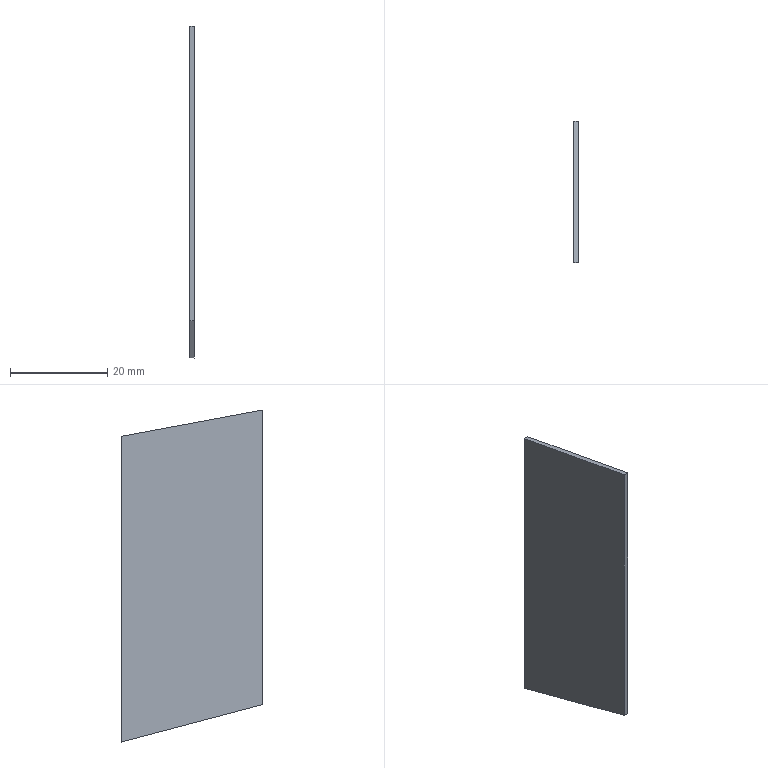Part | STEP file | 09-23 Inlet upper seal plate | 1 solid | 6 faces | box 1 x 29 x 68.181 mm | volume 1787 mm3 | plane 6
STEP:
#1=CARTESIAN_POINT('',(0.,0.,0.));
#2=DIRECTION('',(0.,0.,1.));
#3=DIRECTION('',(1.,0.,0.));
#4=AXIS2_PLACEMENT_3D('',#1,#2,#3);
#5=CARTESIAN_POINT('',(0.,0.,-60.5));
#6=VERTEX_POINT('',#5);
#7=CARTESIAN_POINT('',(1.,0.,-60.5));
#8=VERTEX_POINT('',#7);
#9=CARTESIAN_POINT('',(0.5,0.,-60.5));
#10=DIRECTION('',(1.,0.,0.));
#11=VECTOR('',#10,1.);
#12=LINE('',#9,#11);
#13=CARTESIAN_POINT('',(0.,0.,-60.5));
#14=DIRECTION('',(0.,1.,0.));
#15=DIRECTION('',(0.,0.,1.));
#16=AXIS2_PLACEMENT_3D('',#13,#14,#15);
#17=PLANE('',#16);
#18=CARTESIAN_POINT('',(0.,0.5));
#19=DIRECTION('',(0.,1.));
#20=VECTOR('',#19,1.);
#21=LINE('',#18,#20);
#22=(GEOMETRIC_REPRESENTATION_CONTEXT(2)PARAMETRIC_REPRESENTATION_CONTEXT()REPRESENTATION_CONTEXT('',''));
#23=DEFINITIONAL_REPRESENTATION('',(#21),#22);
#24=PCURVE('',#17,#23);
#25=CARTESIAN_POINT('',(0.,29.,-68.181));
#26=DIRECTION('',(0.,0.256,0.9667));
#27=DIRECTION('',(0.,-0.9667,0.256));
#28=AXIS2_PLACEMENT_3D('',#25,#26,#27);
#29=PLANE('',#28);
#30=CARTESIAN_POINT('',(30.,0.5));
#31=DIRECTION('',(0.,1.));
#32=VECTOR('',#31,1.);
#33=LINE('',#30,#32);
#34=(GEOMETRIC_REPRESENTATION_CONTEXT(2)PARAMETRIC_REPRESENTATION_CONTEXT()REPRESENTATION_CONTEXT('',''));
#35=DEFINITIONAL_REPRESENTATION('',(#33),#34);
#36=PCURVE('',#29,#35);
#37=SURFACE_CURVE('',#12,(#24,#36),.PCURVE_S1.);
#38=EDGE_CURVE('',#6,#8,#37,.T.);
#39=ORIENTED_EDGE('',*,*,#38,.T.);
#40=CARTESIAN_POINT('',(1.,0.,0.));
#41=VERTEX_POINT('',#40);
#42=CARTESIAN_POINT('',(1.,0.,-30.25));
#43=DIRECTION('',(0.,0.,-1.));
#44=VECTOR('',#43,1.);
#45=LINE('',#42,#44);
#46=CARTESIAN_POINT('',(30.25,1.));
#47=DIRECTION('',(-1.,0.));
#48=VECTOR('',#47,1.);
#49=LINE('',#46,#48);
#50=(GEOMETRIC_REPRESENTATION_CONTEXT(2)PARAMETRIC_REPRESENTATION_CONTEXT()REPRESENTATION_CONTEXT('',''));
#51=DEFINITIONAL_REPRESENTATION('',(#49),#50);
#52=PCURVE('',#17,#51);
#53=CARTESIAN_POINT('',(1.,0.,-68.59));
#54=DIRECTION('',(-1.,0.,0.));
#55=DIRECTION('',(0.,0.,1.));
#56=AXIS2_PLACEMENT_3D('',#53,#54,#55);
#57=PLANE('',#56);
#58=CARTESIAN_POINT('',(38.34,0.));
#59=DIRECTION('',(-1.,0.));
#60=VECTOR('',#59,1.);
#61=LINE('',#58,#60);
#62=(GEOMETRIC_REPRESENTATION_CONTEXT(2)PARAMETRIC_REPRESENTATION_CONTEXT()REPRESENTATION_CONTEXT('',''));
#63=DEFINITIONAL_REPRESENTATION('',(#61),#62);
#64=PCURVE('',#57,#63);
#65=SURFACE_CURVE('',#45,(#52,#64),.PCURVE_S1.);
#66=EDGE_CURVE('',#41,#8,#65,.T.);
#67=ORIENTED_EDGE('',*,*,#66,.F.);
#68=CARTESIAN_POINT('',(0.,0.,-0.000000009));
#69=VERTEX_POINT('',#68);
#70=CARTESIAN_POINT('',(0.5,0.,0.));
#71=DIRECTION('',(-1.,0.,0.));
#72=VECTOR('',#71,1.);
#73=LINE('',#70,#72);
#74=CARTESIAN_POINT('',(60.5,0.5));
#75=DIRECTION('',(0.,-1.));
#76=VECTOR('',#75,1.);
#77=LINE('',#74,#76);
#78=(GEOMETRIC_REPRESENTATION_CONTEXT(2)PARAMETRIC_REPRESENTATION_CONTEXT()REPRESENTATION_CONTEXT('',''));
#79=DEFINITIONAL_REPRESENTATION('',(#77),#78);
#80=PCURVE('',#17,#79);
#81=CARTESIAN_POINT('',(0.,0.,0.));
#82=DIRECTION('',(0.,-0.1833,-0.9831));
#83=DIRECTION('',(0.,0.9831,-0.1833));
#84=AXIS2_PLACEMENT_3D('',#81,#82,#83);
#85=PLANE('',#84);
#86=CARTESIAN_POINT('',(0.,0.5));
#87=DIRECTION('',(0.,-1.));
#88=VECTOR('',#87,1.);
#89=LINE('',#86,#88);
#90=(GEOMETRIC_REPRESENTATION_CONTEXT(2)PARAMETRIC_REPRESENTATION_CONTEXT()REPRESENTATION_CONTEXT('',''));
#91=DEFINITIONAL_REPRESENTATION('',(#89),#90);
#92=PCURVE('',#85,#91);
#93=SURFACE_CURVE('',#73,(#80,#92),.PCURVE_S1.);
#94=EDGE_CURVE('',#41,#69,#93,.T.);
#95=ORIENTED_EDGE('',*,*,#94,.T.);
#96=CARTESIAN_POINT('',(0.,0.,-30.25));
#97=DIRECTION('',(0.,0.,1.));
#98=VECTOR('',#97,1.);
#99=LINE('',#96,#98);
#100=CARTESIAN_POINT('',(30.25,0.));
#101=DIRECTION('',(1.,0.));
#102=VECTOR('',#101,1.);
#103=LINE('',#100,#102);
#104=(GEOMETRIC_REPRESENTATION_CONTEXT(2)PARAMETRIC_REPRESENTATION_CONTEXT()REPRESENTATION_CONTEXT('',''));
#105=DEFINITIONAL_REPRESENTATION('',(#103),#104);
#106=PCURVE('',#17,#105);
#107=CARTESIAN_POINT('',(0.,0.,-68.59));
#108=DIRECTION('',(-1.,0.,0.));
#109=DIRECTION('',(0.,0.,1.));
#110=AXIS2_PLACEMENT_3D('',#107,#108,#109);
#111=PLANE('',#110);
#112=CARTESIAN_POINT('',(38.34,0.));
#113=DIRECTION('',(1.,0.));
#114=VECTOR('',#113,1.);
#115=LINE('',#112,#114);
#116=(GEOMETRIC_REPRESENTATION_CONTEXT(2)PARAMETRIC_REPRESENTATION_CONTEXT()REPRESENTATION_CONTEXT('',''));
#117=DEFINITIONAL_REPRESENTATION('',(#115),#116);
#118=PCURVE('',#111,#117);
#119=SURFACE_CURVE('',#99,(#106,#118),.PCURVE_S1.);
#120=EDGE_CURVE('',#6,#69,#119,.T.);
#121=ORIENTED_EDGE('',*,*,#120,.F.);
#122=EDGE_LOOP('',(#39,#67,#95,#121));
#123=FACE_BOUND('',#122,.T.);
#124=ADVANCED_FACE('',(#123),#17,.F.);
#125=CARTESIAN_POINT('',(0.,29.,-5.408));
#126=VERTEX_POINT('',#125);
#127=CARTESIAN_POINT('',(0.,29.,-68.181));
#128=VERTEX_POINT('',#127);
#129=CARTESIAN_POINT('',(0.,29.,-34.091));
#130=DIRECTION('',(0.,0.,-1.));
#131=VECTOR('',#130,1.);
#132=LINE('',#129,#131);
#133=CARTESIAN_POINT('',(34.5,29.));
#134=DIRECTION('',(-1.,0.));
#135=VECTOR('',#134,1.);
#136=LINE('',#133,#135);
#137=(GEOMETRIC_REPRESENTATION_CONTEXT(2)PARAMETRIC_REPRESENTATION_CONTEXT()REPRESENTATION_CONTEXT('',''));
#138=DEFINITIONAL_REPRESENTATION('',(#136),#137);
#139=PCURVE('',#111,#138);
#140=CARTESIAN_POINT('',(0.,29.,-5.408));
#141=DIRECTION('',(0.,-1.,0.));
#142=DIRECTION('',(0.,0.,-1.));
#143=AXIS2_PLACEMENT_3D('',#140,#141,#142);
#144=PLANE('',#143);
#145=CARTESIAN_POINT('',(28.682,0.));
#146=DIRECTION('',(1.,0.));
#147=VECTOR('',#146,1.);
#148=LINE('',#145,#147);
#149=(GEOMETRIC_REPRESENTATION_CONTEXT(2)PARAMETRIC_REPRESENTATION_CONTEXT()REPRESENTATION_CONTEXT('',''));
#150=DEFINITIONAL_REPRESENTATION('',(#148),#149);
#151=PCURVE('',#144,#150);
#152=SURFACE_CURVE('',#132,(#139,#151),.PCURVE_S1.);
#153=EDGE_CURVE('',#126,#128,#152,.T.);
#154=ORIENTED_EDGE('',*,*,#153,.T.);
#155=CARTESIAN_POINT('',(0.,29.,-68.181));
#156=DIRECTION('',(0.,-0.9667,0.256));
#157=VECTOR('',#156,1.);
#158=LINE('',#155,#157);
#159=CARTESIAN_POINT('',(0.4091,29.));
#160=DIRECTION('',(0.256,-0.9667));
#161=VECTOR('',#160,1.);
#162=LINE('',#159,#161);
#163=(GEOMETRIC_REPRESENTATION_CONTEXT(2)PARAMETRIC_REPRESENTATION_CONTEXT()REPRESENTATION_CONTEXT('',''));
#164=DEFINITIONAL_REPRESENTATION('',(#162),#163);
#165=PCURVE('',#111,#164);
#166=CARTESIAN_POINT('',(0.000000004,0.));
#167=DIRECTION('',(1.,0.));
#168=VECTOR('',#167,1.);
#169=LINE('',#166,#168);
#170=(GEOMETRIC_REPRESENTATION_CONTEXT(2)PARAMETRIC_REPRESENTATION_CONTEXT()REPRESENTATION_CONTEXT('',''));
#171=DEFINITIONAL_REPRESENTATION('',(#169),#170);
#172=PCURVE('',#29,#171);
#173=SURFACE_CURVE('',#158,(#165,#172),.PCURVE_S1.);
#174=EDGE_CURVE('',#128,#6,#173,.T.);
#175=ORIENTED_EDGE('',*,*,#174,.T.);
#176=ORIENTED_EDGE('',*,*,#120,.T.);
#177=CARTESIAN_POINT('',(0.,0.,-0.000000017));
#178=DIRECTION('',(0.,0.9831,-0.1833));
#179=VECTOR('',#178,1.);
#180=LINE('',#177,#179);
#181=CARTESIAN_POINT('',(68.59,0.));
#182=DIRECTION('',(-0.1833,0.9831));
#183=VECTOR('',#182,1.);
#184=LINE('',#181,#183);
#185=(GEOMETRIC_REPRESENTATION_CONTEXT(2)PARAMETRIC_REPRESENTATION_CONTEXT()REPRESENTATION_CONTEXT('',''));
#186=DEFINITIONAL_REPRESENTATION('',(#184),#185);
#187=PCURVE('',#111,#186);
#188=CARTESIAN_POINT('',(0.000000003,0.));
#189=DIRECTION('',(1.,0.));
#190=VECTOR('',#189,1.);
#191=LINE('',#188,#190);
#192=(GEOMETRIC_REPRESENTATION_CONTEXT(2)PARAMETRIC_REPRESENTATION_CONTEXT()REPRESENTATION_CONTEXT('',''));
#193=DEFINITIONAL_REPRESENTATION('',(#191),#192);
#194=PCURVE('',#85,#193);
#195=SURFACE_CURVE('',#180,(#187,#194),.PCURVE_S1.);
#196=EDGE_CURVE('',#69,#126,#195,.T.);
#197=ORIENTED_EDGE('',*,*,#196,.T.);
#198=EDGE_LOOP('',(#154,#175,#176,#197));
#199=FACE_BOUND('',#198,.T.);
#200=ADVANCED_FACE('',(#199),#111,.T.);
#201=CARTESIAN_POINT('',(1.,29.,-68.181));
#202=VERTEX_POINT('',#201);
#203=CARTESIAN_POINT('',(1.,29.,-68.181));
#204=DIRECTION('',(0.,-0.9667,0.256));
#205=VECTOR('',#204,1.);
#206=LINE('',#203,#205);
#207=CARTESIAN_POINT('',(0.4091,29.));
#208=DIRECTION('',(0.256,-0.9667));
#209=VECTOR('',#208,1.);
#210=LINE('',#207,#209);
#211=(GEOMETRIC_REPRESENTATION_CONTEXT(2)PARAMETRIC_REPRESENTATION_CONTEXT()REPRESENTATION_CONTEXT('',''));
#212=DEFINITIONAL_REPRESENTATION('',(#210),#211);
#213=PCURVE('',#57,#212);
#214=CARTESIAN_POINT('',(0.,1.));
#215=DIRECTION('',(1.,0.));
#216=VECTOR('',#215,1.);
#217=LINE('',#214,#216);
#218=(GEOMETRIC_REPRESENTATION_CONTEXT(2)PARAMETRIC_REPRESENTATION_CONTEXT()REPRESENTATION_CONTEXT('',''));
#219=DEFINITIONAL_REPRESENTATION('',(#217),#218);
#220=PCURVE('',#29,#219);
#221=SURFACE_CURVE('',#206,(#213,#220),.PCURVE_S1.);
#222=EDGE_CURVE('',#202,#8,#221,.T.);
#223=ORIENTED_EDGE('',*,*,#222,.F.);
#224=CARTESIAN_POINT('',(1.,29.,-5.408));
#225=VERTEX_POINT('',#224);
#226=CARTESIAN_POINT('',(1.,29.,-34.091));
#227=DIRECTION('',(0.,0.,-1.));
#228=VECTOR('',#227,1.);
#229=LINE('',#226,#228);
#230=CARTESIAN_POINT('',(34.5,29.));
#231=DIRECTION('',(-1.,0.));
#232=VECTOR('',#231,1.);
#233=LINE('',#230,#232);
#234=(GEOMETRIC_REPRESENTATION_CONTEXT(2)PARAMETRIC_REPRESENTATION_CONTEXT()REPRESENTATION_CONTEXT('',''));
#235=DEFINITIONAL_REPRESENTATION('',(#233),#234);
#236=PCURVE('',#57,#235);
#237=CARTESIAN_POINT('',(28.682,1.));
#238=DIRECTION('',(1.,0.));
#239=VECTOR('',#238,1.);
#240=LINE('',#237,#239);
#241=(GEOMETRIC_REPRESENTATION_CONTEXT(2)PARAMETRIC_REPRESENTATION_CONTEXT()REPRESENTATION_CONTEXT('',''));
#242=DEFINITIONAL_REPRESENTATION('',(#240),#241);
#243=PCURVE('',#144,#242);
#244=SURFACE_CURVE('',#229,(#236,#243),.PCURVE_S1.);
#245=EDGE_CURVE('',#225,#202,#244,.T.);
#246=ORIENTED_EDGE('',*,*,#245,.F.);
#247=CARTESIAN_POINT('',(1.,0.,0.));
#248=DIRECTION('',(0.,0.9831,-0.1833));
#249=VECTOR('',#248,1.);
#250=LINE('',#247,#249);
#251=CARTESIAN_POINT('',(68.59,0.));
#252=DIRECTION('',(-0.1833,0.9831));
#253=VECTOR('',#252,1.);
#254=LINE('',#251,#253);
#255=(GEOMETRIC_REPRESENTATION_CONTEXT(2)PARAMETRIC_REPRESENTATION_CONTEXT()REPRESENTATION_CONTEXT('',''));
#256=DEFINITIONAL_REPRESENTATION('',(#254),#255);
#257=PCURVE('',#57,#256);
#258=CARTESIAN_POINT('',(0.,1.));
#259=DIRECTION('',(1.,0.));
#260=VECTOR('',#259,1.);
#261=LINE('',#258,#260);
#262=(GEOMETRIC_REPRESENTATION_CONTEXT(2)PARAMETRIC_REPRESENTATION_CONTEXT()REPRESENTATION_CONTEXT('',''));
#263=DEFINITIONAL_REPRESENTATION('',(#261),#262);
#264=PCURVE('',#85,#263);
#265=SURFACE_CURVE('',#250,(#257,#264),.PCURVE_S1.);
#266=EDGE_CURVE('',#41,#225,#265,.T.);
#267=ORIENTED_EDGE('',*,*,#266,.F.);
#268=ORIENTED_EDGE('',*,*,#66,.T.);
#269=EDGE_LOOP('',(#223,#246,#267,#268));
#270=FACE_BOUND('',#269,.T.);
#271=ADVANCED_FACE('',(#270),#57,.F.);
#272=CARTESIAN_POINT('',(0.5,29.,-68.181));
#273=DIRECTION('',(-1.,0.,0.));
#274=VECTOR('',#273,1.);
#275=LINE('',#272,#274);
#276=CARTESIAN_POINT('',(0.,0.5));
#277=DIRECTION('',(0.,-1.));
#278=VECTOR('',#277,1.);
#279=LINE('',#276,#278);
#280=(GEOMETRIC_REPRESENTATION_CONTEXT(2)PARAMETRIC_REPRESENTATION_CONTEXT()REPRESENTATION_CONTEXT('',''));
#281=DEFINITIONAL_REPRESENTATION('',(#279),#280);
#282=PCURVE('',#29,#281);
#283=CARTESIAN_POINT('',(62.773,0.5));
#284=DIRECTION('',(0.,-1.));
#285=VECTOR('',#284,1.);
#286=LINE('',#283,#285);
#287=(GEOMETRIC_REPRESENTATION_CONTEXT(2)PARAMETRIC_REPRESENTATION_CONTEXT()REPRESENTATION_CONTEXT('',''));
#288=DEFINITIONAL_REPRESENTATION('',(#286),#287);
#289=PCURVE('',#144,#288);
#290=SURFACE_CURVE('',#275,(#282,#289),.PCURVE_S1.);
#291=EDGE_CURVE('',#202,#128,#290,.T.);
#292=ORIENTED_EDGE('',*,*,#291,.F.);
#293=ORIENTED_EDGE('',*,*,#222,.T.);
#294=ORIENTED_EDGE('',*,*,#38,.F.);
#295=ORIENTED_EDGE('',*,*,#174,.F.);
#296=EDGE_LOOP('',(#292,#293,#294,#295));
#297=FACE_BOUND('',#296,.T.);
#298=ADVANCED_FACE('',(#297),#29,.F.);
#299=CARTESIAN_POINT('',(0.5,29.,-5.408));
#300=DIRECTION('',(-1.,0.,0.));
#301=VECTOR('',#300,1.);
#302=LINE('',#299,#301);
#303=CARTESIAN_POINT('',(0.,0.5));
#304=DIRECTION('',(0.,-1.));
#305=VECTOR('',#304,1.);
#306=LINE('',#303,#305);
#307=(GEOMETRIC_REPRESENTATION_CONTEXT(2)PARAMETRIC_REPRESENTATION_CONTEXT()REPRESENTATION_CONTEXT('',''));
#308=DEFINITIONAL_REPRESENTATION('',(#306),#307);
#309=PCURVE('',#144,#308);
#310=CARTESIAN_POINT('',(29.5,0.5));
#311=DIRECTION('',(0.,-1.));
#312=VECTOR('',#311,1.);
#313=LINE('',#310,#312);
#314=(GEOMETRIC_REPRESENTATION_CONTEXT(2)PARAMETRIC_REPRESENTATION_CONTEXT()REPRESENTATION_CONTEXT('',''));
#315=DEFINITIONAL_REPRESENTATION('',(#313),#314);
#316=PCURVE('',#85,#315);
#317=SURFACE_CURVE('',#302,(#309,#316),.PCURVE_S1.);
#318=EDGE_CURVE('',#225,#126,#317,.T.);
#319=ORIENTED_EDGE('',*,*,#318,.F.);
#320=ORIENTED_EDGE('',*,*,#245,.T.);
#321=ORIENTED_EDGE('',*,*,#291,.T.);
#322=ORIENTED_EDGE('',*,*,#153,.F.);
#323=EDGE_LOOP('',(#319,#320,#321,#322));
#324=FACE_BOUND('',#323,.T.);
#325=ADVANCED_FACE('',(#324),#144,.F.);
#326=ORIENTED_EDGE('',*,*,#94,.F.);
#327=ORIENTED_EDGE('',*,*,#266,.T.);
#328=ORIENTED_EDGE('',*,*,#318,.T.);
#329=ORIENTED_EDGE('',*,*,#196,.F.);
#330=EDGE_LOOP('',(#326,#327,#328,#329));
#331=FACE_BOUND('',#330,.T.);
#332=ADVANCED_FACE('',(#331),#85,.F.);
#333=CLOSED_SHELL('',(#124,#200,#271,#298,#325,#332));
#334=MANIFOLD_SOLID_BREP('',#333);
#335=(LENGTH_UNIT()NAMED_UNIT(*)SI_UNIT(.MILLI.,.METRE.));
#336=UNCERTAINTY_MEASURE_WITH_UNIT(LENGTH_MEASURE(0.0000001),#335,'','');
#337=(NAMED_UNIT(*)PLANE_ANGLE_UNIT()SI_UNIT($,.RADIAN.));
#338=(NAMED_UNIT(*)SI_UNIT($,.STERADIAN.)SOLID_ANGLE_UNIT());
#339=(GEOMETRIC_REPRESENTATION_CONTEXT(3)GLOBAL_UNCERTAINTY_ASSIGNED_CONTEXT((#336))GLOBAL_UNIT_ASSIGNED_CONTEXT((#335,#337,#338))REPRESENTATION_CONTEXT('',''));
#340=ADVANCED_BREP_SHAPE_REPRESENTATION('',(#4,#334),#339);